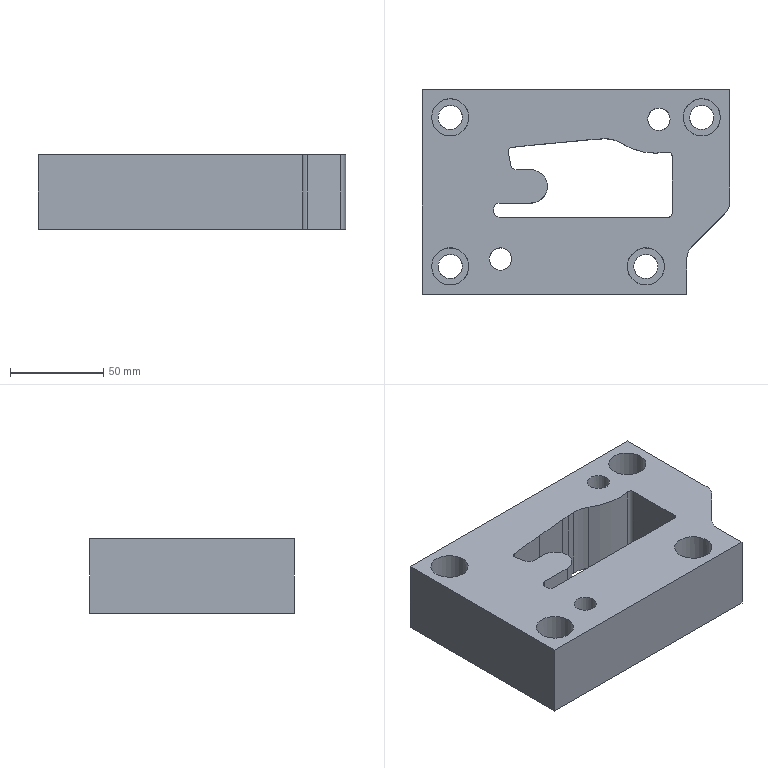Part | STEP file | gslz 2016.10.28-13_id482_x_t | 1 solid | 44 faces | box 165 x 110 x 40 mm | volume 527172 mm3 | plane 22 | cylinder 22 | commonest cylinder face diameters 13 x4 20 x4 4 x3 6 x3 18 x3 12 x2